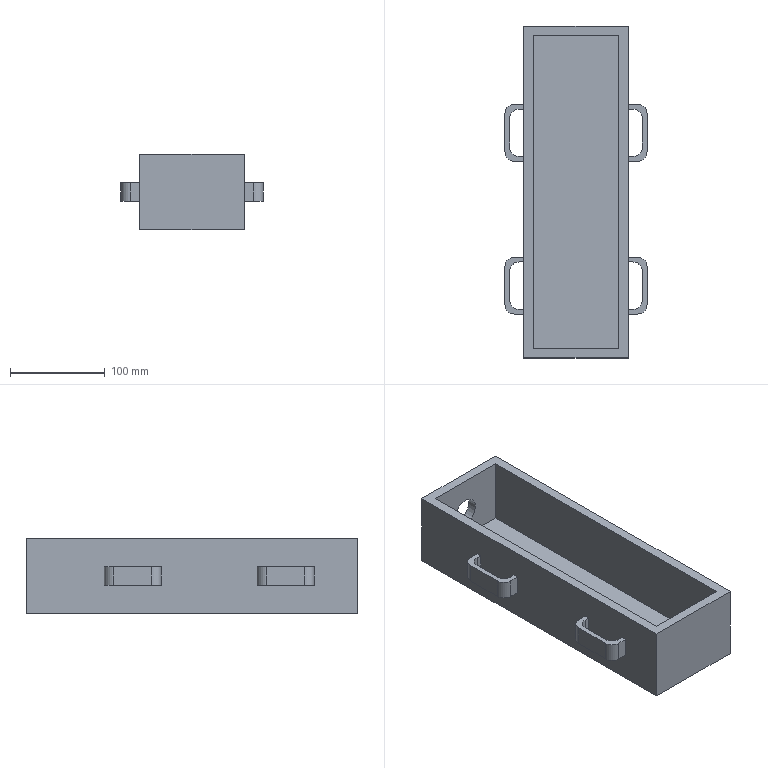Part | SolidWorks | features Cut 2, Extrusion 1, Fillet 1, ICE 1, MirrorPattern 1, Shell 1 | 1 solid | 61 faces | box 150 x 350 x 80 mm | volume 1029931 mm3 | plane 43 | cylinder 18 | commonest cylinder face diameters 20 x16 30 x2